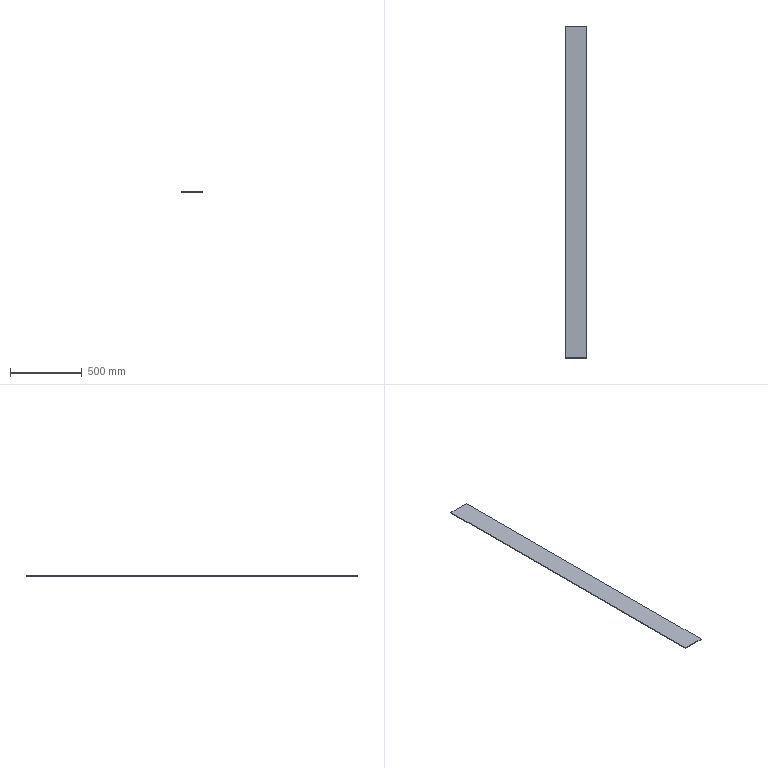Part | SolidWorks | features Extrusion 1, HoleWzd 1 | 1 solid | 6 faces | box 151 x 2310 x 5 mm | volume 1744050 mm3 | plane 6
STEP:
#1=CARTESIAN_POINT('',(75.5,-1155.,0.));
#2=VERTEX_POINT('',#1);
#3=CARTESIAN_POINT('',(75.5,1155.,0.));
#4=VERTEX_POINT('',#3);
#5=CARTESIAN_POINT('',(75.5,1155.,0.));
#6=DIRECTION('',(0.,1.,0.));
#7=VECTOR('',#6,1000.);
#8=LINE('',#5,#7);
#9=EDGE_CURVE('',#2,#4,#8,.T.);
#10=ORIENTED_EDGE('',*,*,#9,.T.);
#11=CARTESIAN_POINT('',(75.5,1155.,5.));
#12=VERTEX_POINT('',#11);
#13=CARTESIAN_POINT('',(75.5,1155.,5.));
#14=DIRECTION('',(0.,0.,-1.));
#15=VECTOR('',#14,1000.);
#16=LINE('',#13,#15);
#17=EDGE_CURVE('',#12,#4,#16,.T.);
#18=ORIENTED_EDGE('',*,*,#17,.F.);
#19=CARTESIAN_POINT('',(75.5,-1155.,5.));
#20=VERTEX_POINT('',#19);
#21=CARTESIAN_POINT('',(75.5,1155.,5.));
#22=DIRECTION('',(0.,1.,0.));
#23=VECTOR('',#22,1000.);
#24=LINE('',#21,#23);
#25=EDGE_CURVE('',#20,#12,#24,.T.);
#26=ORIENTED_EDGE('',*,*,#25,.F.);
#27=CARTESIAN_POINT('',(75.5,-1155.,5.));
#28=DIRECTION('',(0.,0.,-1.));
#29=VECTOR('',#28,1000.);
#30=LINE('',#27,#29);
#31=EDGE_CURVE('',#20,#2,#30,.T.);
#32=ORIENTED_EDGE('',*,*,#31,.T.);
#33=EDGE_LOOP('',(#10,#18,#26,#32));
#34=FACE_OUTER_BOUND('',#33,.T.);
#35=CARTESIAN_POINT('',(75.5,1155.,5.));
#36=DIRECTION('',(-1.,0.,0.));
#37=DIRECTION('',(0.,-1.,0.));
#38=AXIS2_PLACEMENT_3D('',#35,#36,#37);
#39=PLANE('',#38);
#40=ADVANCED_FACE('',(#34),#39,.F.);
#41=CARTESIAN_POINT('',(-75.5,1155.,0.));
#42=VERTEX_POINT('',#41);
#43=CARTESIAN_POINT('',(-75.5,1155.,0.));
#44=DIRECTION('',(-1.,0.,0.));
#45=VECTOR('',#44,1000.);
#46=LINE('',#43,#45);
#47=EDGE_CURVE('',#4,#42,#46,.T.);
#48=ORIENTED_EDGE('',*,*,#47,.T.);
#49=CARTESIAN_POINT('',(-75.5,1155.,5.));
#50=VERTEX_POINT('',#49);
#51=CARTESIAN_POINT('',(-75.5,1155.,5.));
#52=DIRECTION('',(0.,0.,-1.));
#53=VECTOR('',#52,1000.);
#54=LINE('',#51,#53);
#55=EDGE_CURVE('',#50,#42,#54,.T.);
#56=ORIENTED_EDGE('',*,*,#55,.F.);
#57=CARTESIAN_POINT('',(-75.5,1155.,5.));
#58=DIRECTION('',(-1.,0.,0.));
#59=VECTOR('',#58,1000.);
#60=LINE('',#57,#59);
#61=EDGE_CURVE('',#12,#50,#60,.T.);
#62=ORIENTED_EDGE('',*,*,#61,.F.);
#63=ORIENTED_EDGE('',*,*,#17,.T.);
#64=EDGE_LOOP('',(#48,#56,#62,#63));
#65=FACE_OUTER_BOUND('',#64,.T.);
#66=CARTESIAN_POINT('',(-75.5,1155.,5.));
#67=DIRECTION('',(0.,-1.,0.));
#68=DIRECTION('',(0.,0.,-1.));
#69=AXIS2_PLACEMENT_3D('',#66,#67,#68);
#70=PLANE('',#69);
#71=ADVANCED_FACE('',(#65),#70,.F.);
#72=CARTESIAN_POINT('',(-75.5,-1155.,0.));
#73=VERTEX_POINT('',#72);
#74=CARTESIAN_POINT('',(-75.5,1155.,0.));
#75=DIRECTION('',(0.,-1.,0.));
#76=VECTOR('',#75,1000.);
#77=LINE('',#74,#76);
#78=EDGE_CURVE('',#42,#73,#77,.T.);
#79=ORIENTED_EDGE('',*,*,#78,.T.);
#80=CARTESIAN_POINT('',(-75.5,-1155.,5.));
#81=VERTEX_POINT('',#80);
#82=CARTESIAN_POINT('',(-75.5,-1155.,5.));
#83=DIRECTION('',(0.,0.,-1.));
#84=VECTOR('',#83,1000.);
#85=LINE('',#82,#84);
#86=EDGE_CURVE('',#81,#73,#85,.T.);
#87=ORIENTED_EDGE('',*,*,#86,.F.);
#88=CARTESIAN_POINT('',(-75.5,1155.,5.));
#89=DIRECTION('',(0.,-1.,0.));
#90=VECTOR('',#89,1000.);
#91=LINE('',#88,#90);
#92=EDGE_CURVE('',#50,#81,#91,.T.);
#93=ORIENTED_EDGE('',*,*,#92,.F.);
#94=ORIENTED_EDGE('',*,*,#55,.T.);
#95=EDGE_LOOP('',(#79,#87,#93,#94));
#96=FACE_OUTER_BOUND('',#95,.T.);
#97=CARTESIAN_POINT('',(-75.5,1155.,5.));
#98=DIRECTION('',(1.,0.,0.));
#99=DIRECTION('',(0.,1.,0.));
#100=AXIS2_PLACEMENT_3D('',#97,#98,#99);
#101=PLANE('',#100);
#102=ADVANCED_FACE('',(#96),#101,.F.);
#103=CARTESIAN_POINT('',(-75.5,-1155.,0.));
#104=DIRECTION('',(1.,0.,0.));
#105=VECTOR('',#104,1000.);
#106=LINE('',#103,#105);
#107=EDGE_CURVE('',#73,#2,#106,.T.);
#108=ORIENTED_EDGE('',*,*,#107,.T.);
#109=ORIENTED_EDGE('',*,*,#31,.F.);
#110=CARTESIAN_POINT('',(-75.5,-1155.,5.));
#111=DIRECTION('',(1.,0.,0.));
#112=VECTOR('',#111,1000.);
#113=LINE('',#110,#112);
#114=EDGE_CURVE('',#81,#20,#113,.T.);
#115=ORIENTED_EDGE('',*,*,#114,.F.);
#116=ORIENTED_EDGE('',*,*,#86,.T.);
#117=EDGE_LOOP('',(#108,#109,#115,#116));
#118=FACE_OUTER_BOUND('',#117,.T.);
#119=CARTESIAN_POINT('',(-75.5,-1155.,5.));
#120=DIRECTION('',(0.,1.,0.));
#121=DIRECTION('',(0.,0.,1.));
#122=AXIS2_PLACEMENT_3D('',#119,#120,#121);
#123=PLANE('',#122);
#124=ADVANCED_FACE('',(#118),#123,.F.);
#125=ORIENTED_EDGE('',*,*,#25,.T.);
#126=ORIENTED_EDGE('',*,*,#61,.T.);
#127=ORIENTED_EDGE('',*,*,#92,.T.);
#128=ORIENTED_EDGE('',*,*,#114,.T.);
#129=EDGE_LOOP('',(#125,#126,#127,#128));
#130=FACE_OUTER_BOUND('',#129,.T.);
#131=CARTESIAN_POINT('',(0.,0.,5.));
#132=DIRECTION('',(0.,0.,1.));
#133=DIRECTION('',(1.,0.,0.));
#134=AXIS2_PLACEMENT_3D('',#131,#132,#133);
#135=PLANE('',#134);
#136=ADVANCED_FACE('',(#130),#135,.T.);
#137=ORIENTED_EDGE('',*,*,#9,.F.);
#138=ORIENTED_EDGE('',*,*,#107,.F.);
#139=ORIENTED_EDGE('',*,*,#78,.F.);
#140=ORIENTED_EDGE('',*,*,#47,.F.);
#141=EDGE_LOOP('',(#137,#138,#139,#140));
#142=FACE_OUTER_BOUND('',#141,.T.);
#143=CARTESIAN_POINT('',(0.,0.,0.));
#144=DIRECTION('',(0.,0.,1.));
#145=DIRECTION('',(1.,0.,0.));
#146=AXIS2_PLACEMENT_3D('',#143,#144,#145);
#147=PLANE('',#146);
#148=ADVANCED_FACE('',(#142),#147,.F.);
#149=CLOSED_SHELL('',(#40,#71,#102,#124,#136,#148));
#150=MANIFOLD_SOLID_BREP('',#149);
#151=CARTESIAN_POINT('',(0.,0.,0.));
#152=DIRECTION('',(0.,0.,1.));
#153=DIRECTION('',(1.,0.,0.));
#154=AXIS2_PLACEMENT_3D('',#151,#152,#153);
#155=(LENGTH_UNIT()NAMED_UNIT(*)SI_UNIT(.MILLI.,.METRE.));
#156=UNCERTAINTY_MEASURE_WITH_UNIT(LENGTH_MEASURE(0.00001),#155,'','');
#157=(NAMED_UNIT(*)PLANE_ANGLE_UNIT()SI_UNIT($,.RADIAN.));
#158=(NAMED_UNIT(*)SI_UNIT($,.STERADIAN.)SOLID_ANGLE_UNIT());
#159=(GEOMETRIC_REPRESENTATION_CONTEXT(3)GLOBAL_UNCERTAINTY_ASSIGNED_CONTEXT((#156))GLOBAL_UNIT_ASSIGNED_CONTEXT((#155,#157,#158))REPRESENTATION_CONTEXT('',''));
#160=ADVANCED_BREP_SHAPE_REPRESENTATION('',(#150,#154),#159);